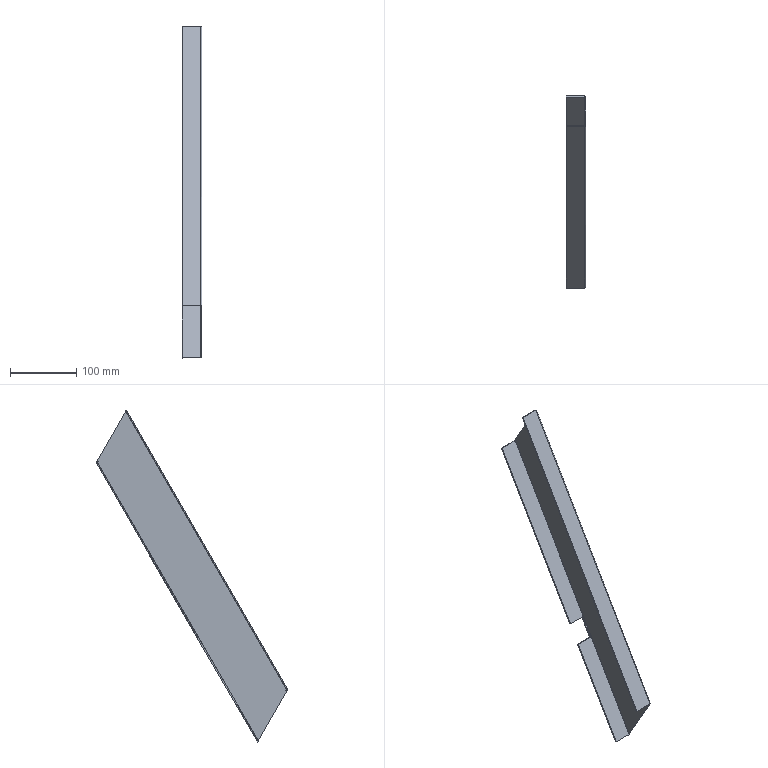Part | STEP file | Guard Rib 2 | 1 solid | 29 faces | box 30 x 290.188 x 502.62 mm | volume 129712 mm3 | plane 20 | cylinder 7 | spline 2 | commonest cylinder face diameters 1 x5 5 x2
STEP:
#1=CARTESIAN_POINT('',(-2.,-21.009,-479.727));
#2=VERTEX_POINT('',#1);
#3=CARTESIAN_POINT('',(-2.,-20.759,-478.794));
#4=VERTEX_POINT('',#3);
#5=CARTESIAN_POINT('',(-2.,-21.009,-479.227));
#6=DIRECTION('',(1.,0.,0.));
#7=DIRECTION('',(0.,0.,-1.));
#8=AXIS2_PLACEMENT_3D('',#5,#6,#7);
#9=CIRCLE('',#8,0.5);
#10=EDGE_CURVE('',#2,#4,#9,.T.);
#11=ORIENTED_EDGE('',*,*,#10,.F.);
#12=CARTESIAN_POINT('',(0.,-21.009,-479.727));
#13=VERTEX_POINT('',#12);
#14=CARTESIAN_POINT('',(-2.,-21.009,-479.727));
#15=DIRECTION('',(1.,0.,0.));
#16=VECTOR('',#15,1000.);
#17=LINE('',#14,#16);
#18=EDGE_CURVE('',#2,#13,#17,.T.);
#19=ORIENTED_EDGE('',*,*,#18,.T.);
#20=CARTESIAN_POINT('',(0.,-20.759,-478.794));
#21=VERTEX_POINT('',#20);
#22=CARTESIAN_POINT('',(0.,-21.009,-479.227));
#23=DIRECTION('',(-1.,0.,0.));
#24=DIRECTION('',(0.,0.,-1.));
#25=AXIS2_PLACEMENT_3D('',#22,#23,#24);
#26=CIRCLE('',#25,0.5);
#27=EDGE_CURVE('',#21,#13,#26,.T.);
#28=ORIENTED_EDGE('',*,*,#27,.F.);
#29=CARTESIAN_POINT('',(-2.,-20.759,-478.794));
#30=DIRECTION('',(1.,0.,0.));
#31=VECTOR('',#30,1000.);
#32=LINE('',#29,#31);
#33=EDGE_CURVE('',#4,#21,#32,.T.);
#34=ORIENTED_EDGE('',*,*,#33,.F.);
#35=EDGE_LOOP('',(#11,#19,#28,#34));
#36=FACE_OUTER_BOUND('',#35,.T.);
#37=CARTESIAN_POINT('',(-2.,-21.009,-479.227));
#38=DIRECTION('',(1.,0.,0.));
#39=DIRECTION('',(0.,0.,-1.));
#40=AXIS2_PLACEMENT_3D('',#37,#38,#39);
#41=CYLINDRICAL_SURFACE('',#40,0.5);
#42=ADVANCED_FACE('',(#36),#41,.F.);
#43=CARTESIAN_POINT('',(0.,-21.625,-478.294));
#44=VERTEX_POINT('',#43);
#45=CARTESIAN_POINT('',(0.,-21.625,-478.294));
#46=DIRECTION('',(0.,-0.866,0.5));
#47=VECTOR('',#46,1000.);
#48=LINE('',#45,#47);
#49=EDGE_CURVE('',#21,#44,#48,.T.);
#50=ORIENTED_EDGE('',*,*,#49,.F.);
#51=ORIENTED_EDGE('',*,*,#27,.T.);
#52=CARTESIAN_POINT('',(0.,-21.259,-479.66));
#53=VERTEX_POINT('',#52);
#54=CARTESIAN_POINT('',(0.,-21.009,-479.227));
#55=DIRECTION('',(-1.,0.,0.));
#56=DIRECTION('',(0.,0.,-1.));
#57=AXIS2_PLACEMENT_3D('',#54,#55,#56);
#58=CIRCLE('',#57,0.5);
#59=EDGE_CURVE('',#13,#53,#58,.T.);
#60=ORIENTED_EDGE('',*,*,#59,.T.);
#61=CARTESIAN_POINT('',(0.,-22.79,-478.776));
#62=VERTEX_POINT('',#61);
#63=CARTESIAN_POINT('',(0.,-22.79,-478.776));
#64=DIRECTION('',(0.,0.866,-0.5));
#65=VECTOR('',#64,1000.);
#66=LINE('',#63,#65);
#67=EDGE_CURVE('',#62,#53,#66,.T.);
#68=ORIENTED_EDGE('',*,*,#67,.F.);
#69=CARTESIAN_POINT('',(0.,20.955,-554.544));
#70=VERTEX_POINT('',#69);
#71=CARTESIAN_POINT('',(0.,20.955,-554.544));
#72=DIRECTION('',(0.,-0.5,0.866));
#73=VECTOR('',#72,1000.);
#74=LINE('',#71,#73);
#75=EDGE_CURVE('',#70,#62,#74,.T.);
#76=ORIENTED_EDGE('',*,*,#75,.F.);
#77=CARTESIAN_POINT('',(0.,264.233,-133.173));
#78=VERTEX_POINT('',#77);
#79=CARTESIAN_POINT('',(0.,264.233,-133.173));
#80=DIRECTION('',(0.,-0.5,-0.866));
#81=VECTOR('',#80,1000.);
#82=LINE('',#79,#81);
#83=EDGE_CURVE('',#78,#70,#82,.T.);
#84=ORIENTED_EDGE('',*,*,#83,.F.);
#85=CARTESIAN_POINT('',(0.,263.367,-132.673));
#86=VERTEX_POINT('',#85);
#87=CARTESIAN_POINT('',(0.,264.233,-133.173));
#88=DIRECTION('',(0.,0.866,-0.5));
#89=VECTOR('',#88,1000.);
#90=LINE('',#87,#89);
#91=EDGE_CURVE('',#86,#78,#90,.T.);
#92=ORIENTED_EDGE('',*,*,#91,.F.);
#93=CARTESIAN_POINT('',(0.,263.867,-131.807));
#94=VERTEX_POINT('',#93);
#95=CARTESIAN_POINT('',(0.,263.617,-132.24));
#96=DIRECTION('',(-1.,0.,0.));
#97=DIRECTION('',(0.,0.,-1.));
#98=AXIS2_PLACEMENT_3D('',#95,#96,#97);
#99=CIRCLE('',#98,0.5);
#100=EDGE_CURVE('',#86,#94,#99,.T.);
#101=ORIENTED_EDGE('',*,*,#100,.T.);
#102=CARTESIAN_POINT('',(0.,265.398,-132.691));
#103=VERTEX_POINT('',#102);
#104=CARTESIAN_POINT('',(0.,265.398,-132.691));
#105=DIRECTION('',(0.,-0.866,0.5));
#106=VECTOR('',#105,1000.);
#107=LINE('',#104,#106);
#108=EDGE_CURVE('',#103,#94,#107,.T.);
#109=ORIENTED_EDGE('',*,*,#108,.F.);
#110=CARTESIAN_POINT('',(0.,221.653,-56.923));
#111=VERTEX_POINT('',#110);
#112=CARTESIAN_POINT('',(0.,221.653,-56.923));
#113=DIRECTION('',(0.,0.5,-0.866));
#114=VECTOR('',#113,1000.);
#115=LINE('',#112,#114);
#116=EDGE_CURVE('',#111,#103,#115,.T.);
#117=ORIENTED_EDGE('',*,*,#116,.F.);
#118=CARTESIAN_POINT('',(0.,-21.625,-478.294));
#119=DIRECTION('',(0.,0.5,0.866));
#120=VECTOR('',#119,1000.);
#121=LINE('',#118,#120);
#122=EDGE_CURVE('',#44,#111,#121,.T.);
#123=ORIENTED_EDGE('',*,*,#122,.F.);
#124=EDGE_LOOP('',(#50,#51,#60,#68,#76,#84,#92,#101,#109,#117,#123));
#125=FACE_OUTER_BOUND('',#124,.T.);
#126=CARTESIAN_POINT('',(0.,0.,0.));
#127=DIRECTION('',(-1.,0.,0.));
#128=DIRECTION('',(0.,0.,1.));
#129=AXIS2_PLACEMENT_3D('',#126,#127,#128);
#130=PLANE('',#129);
#131=ADVANCED_FACE('',(#125),#130,.F.);
#132=CARTESIAN_POINT('',(-2.5,220.21,-54.423));
#133=VERTEX_POINT('',#132);
#134=CARTESIAN_POINT('',(-2.5,-23.79,-477.044));
#135=VERTEX_POINT('',#134);
#136=CARTESIAN_POINT('',(-2.5,220.21,-54.423));
#137=DIRECTION('',(0.,-0.5,-0.866));
#138=VECTOR('',#137,1000.);
#139=LINE('',#136,#138);
#140=EDGE_CURVE('',#133,#135,#139,.T.);
#141=ORIENTED_EDGE('',*,*,#140,.T.);
#142=CARTESIAN_POINT('',(-2.5,-21.625,-478.294));
#143=DIRECTION('',(0.,0.5,0.866));
#144=DIRECTION('',(0.,-0.866,0.5));
#145=AXIS2_PLACEMENT_3D('',#142,#143,#144);
#146=CIRCLE('',#145,2.5);
#147=EDGE_CURVE('',#135,#44,#146,.T.);
#148=ORIENTED_EDGE('',*,*,#147,.T.);
#149=ORIENTED_EDGE('',*,*,#122,.T.);
#150=CARTESIAN_POINT('',(0.,221.653,-56.923));
#151=CARTESIAN_POINT('',(0.,221.428,-56.653));
#152=CARTESIAN_POINT('',(-0.0634,221.21,-56.392));
#153=CARTESIAN_POINT('',(-0.2525,220.905,-56.005));
#154=CARTESIAN_POINT('',(-0.3297,220.81,-55.881));
#155=CARTESIAN_POINT('',(-0.5105,220.635,-55.642));
#156=CARTESIAN_POINT('',(-0.6149,220.555,-55.526));
#157=CARTESIAN_POINT('',(-0.8474,220.414,-55.305));
#158=CARTESIAN_POINT('',(-0.9735,220.354,-55.201));
#159=CARTESIAN_POINT('',(-1.244,220.257,-55.007));
#160=CARTESIAN_POINT('',(-1.391,220.219,-54.915));
#161=CARTESIAN_POINT('',(-1.693,220.17,-54.748));
#162=CARTESIAN_POINT('',(-1.849,220.159,-54.673));
#163=CARTESIAN_POINT('',(-2.17,220.164,-54.537));
#164=CARTESIAN_POINT('',(-2.335,220.18,-54.476));
#165=CARTESIAN_POINT('',(-2.5,220.21,-54.423));
#166=B_SPLINE_CURVE_WITH_KNOTS('',3,(#150,#151,#152,#153,#154,#155,#156,#157,#158,#159,#160,#161,#162,#163,#164,#165),.UNSPECIFIED.,.F.,.F.,(4,2,2,2,2,2,2,4),(0.,0.001038,0.001557,0.002076,0.002595,0.003114,0.003633,0.004151),.UNSPECIFIED.);
#167=EDGE_CURVE('',#111,#133,#166,.T.);
#168=ORIENTED_EDGE('',*,*,#167,.T.);
#169=EDGE_LOOP('',(#141,#148,#149,#168));
#170=FACE_OUTER_BOUND('',#169,.T.);
#171=CARTESIAN_POINT('',(-2.5,222.375,-55.673));
#172=DIRECTION('',(0.,0.5,0.866));
#173=DIRECTION('',(0.,-0.866,0.5));
#174=AXIS2_PLACEMENT_3D('',#171,#172,#173);
#175=CYLINDRICAL_SURFACE('',#174,2.5);
#176=ADVANCED_FACE('',(#170),#175,.T.);
#177=CARTESIAN_POINT('',(-2.,-21.259,-479.66));
#178=VERTEX_POINT('',#177);
#179=CARTESIAN_POINT('',(-2.,-21.259,-479.66));
#180=DIRECTION('',(-1.,0.,0.));
#181=VECTOR('',#180,1000.);
#182=LINE('',#179,#181);
#183=EDGE_CURVE('',#53,#178,#182,.T.);
#184=ORIENTED_EDGE('',*,*,#183,.T.);
#185=CARTESIAN_POINT('',(-2.,-22.79,-478.776));
#186=VERTEX_POINT('',#185);
#187=CARTESIAN_POINT('',(-2.,-21.259,-479.66));
#188=DIRECTION('',(0.,-0.866,0.5));
#189=VECTOR('',#188,1000.);
#190=LINE('',#187,#189);
#191=EDGE_CURVE('',#178,#186,#190,.T.);
#192=ORIENTED_EDGE('',*,*,#191,.T.);
#193=CARTESIAN_POINT('',(-2.,-22.79,-478.776));
#194=DIRECTION('',(1.,0.,0.));
#195=VECTOR('',#194,1000.);
#196=LINE('',#193,#195);
#197=EDGE_CURVE('',#186,#62,#196,.T.);
#198=ORIENTED_EDGE('',*,*,#197,.T.);
#199=ORIENTED_EDGE('',*,*,#67,.T.);
#200=EDGE_LOOP('',(#184,#192,#198,#199));
#201=FACE_OUTER_BOUND('',#200,.T.);
#202=CARTESIAN_POINT('',(-2.,-21.259,-479.66));
#203=DIRECTION('',(0.,0.5,0.866));
#204=DIRECTION('',(0.,-0.866,0.5));
#205=AXIS2_PLACEMENT_3D('',#202,#203,#204);
#206=PLANE('',#205);
#207=ADVANCED_FACE('',(#201),#206,.T.);
#208=CARTESIAN_POINT('',(-2.,20.955,-554.544));
#209=VERTEX_POINT('',#208);
#210=CARTESIAN_POINT('',(-2.,-23.79,-477.044));
#211=DIRECTION('',(0.,0.5,-0.866));
#212=VECTOR('',#211,1000.);
#213=LINE('',#210,#212);
#214=EDGE_CURVE('',#186,#209,#213,.T.);
#215=ORIENTED_EDGE('',*,*,#214,.T.);
#216=CARTESIAN_POINT('',(-2.,20.955,-554.544));
#217=DIRECTION('',(1.,0.,0.));
#218=VECTOR('',#217,1000.);
#219=LINE('',#216,#218);
#220=EDGE_CURVE('',#209,#70,#219,.T.);
#221=ORIENTED_EDGE('',*,*,#220,.T.);
#222=ORIENTED_EDGE('',*,*,#75,.T.);
#223=ORIENTED_EDGE('',*,*,#197,.F.);
#224=EDGE_LOOP('',(#215,#221,#222,#223));
#225=FACE_OUTER_BOUND('',#224,.T.);
#226=CARTESIAN_POINT('',(-2.,-23.79,-477.044));
#227=DIRECTION('',(0.,-0.866,-0.5));
#228=DIRECTION('',(0.,0.5,-0.866));
#229=AXIS2_PLACEMENT_3D('',#226,#227,#228);
#230=PLANE('',#229);
#231=ADVANCED_FACE('',(#225),#230,.T.);
#232=CARTESIAN_POINT('',(-2.5,22.398,-557.044));
#233=VERTEX_POINT('',#232);
#234=CARTESIAN_POINT('',(-2.5,266.398,-134.423));
#235=VERTEX_POINT('',#234);
#236=CARTESIAN_POINT('',(-2.5,22.398,-557.044));
#237=DIRECTION('',(0.,0.5,0.866));
#238=VECTOR('',#237,1000.);
#239=LINE('',#236,#238);
#240=EDGE_CURVE('',#233,#235,#239,.T.);
#241=ORIENTED_EDGE('',*,*,#240,.T.);
#242=CARTESIAN_POINT('',(-2.5,264.233,-133.173));
#243=DIRECTION('',(0.,-0.5,-0.866));
#244=DIRECTION('',(0.,0.866,-0.5));
#245=AXIS2_PLACEMENT_3D('',#242,#243,#244);
#246=CIRCLE('',#245,2.5);
#247=EDGE_CURVE('',#235,#78,#246,.T.);
#248=ORIENTED_EDGE('',*,*,#247,.T.);
#249=ORIENTED_EDGE('',*,*,#83,.T.);
#250=CARTESIAN_POINT('',(0.,20.955,-554.544));
#251=CARTESIAN_POINT('',(0.,21.18,-554.814));
#252=CARTESIAN_POINT('',(-0.0634,21.398,-555.075));
#253=CARTESIAN_POINT('',(-0.2525,21.703,-555.462));
#254=CARTESIAN_POINT('',(-0.3297,21.798,-555.586));
#255=CARTESIAN_POINT('',(-0.5105,21.973,-555.825));
#256=CARTESIAN_POINT('',(-0.6149,22.054,-555.941));
#257=CARTESIAN_POINT('',(-0.8474,22.195,-556.162));
#258=CARTESIAN_POINT('',(-0.9735,22.255,-556.265));
#259=CARTESIAN_POINT('',(-1.244,22.352,-556.46));
#260=CARTESIAN_POINT('',(-1.391,22.389,-556.552));
#261=CARTESIAN_POINT('',(-1.693,22.438,-556.719));
#262=CARTESIAN_POINT('',(-1.849,22.449,-556.794));
#263=CARTESIAN_POINT('',(-2.17,22.445,-556.93));
#264=CARTESIAN_POINT('',(-2.335,22.428,-556.991));
#265=CARTESIAN_POINT('',(-2.5,22.398,-557.044));
#266=B_SPLINE_CURVE_WITH_KNOTS('',3,(#250,#251,#252,#253,#254,#255,#256,#257,#258,#259,#260,#261,#262,#263,#264,#265),.UNSPECIFIED.,.F.,.F.,(4,2,2,2,2,2,2,4),(0.,0.001038,0.001557,0.002076,0.002595,0.003114,0.003633,0.004151),.UNSPECIFIED.);
#267=EDGE_CURVE('',#70,#233,#266,.T.);
#268=ORIENTED_EDGE('',*,*,#267,.T.);
#269=EDGE_LOOP('',(#241,#248,#249,#268));
#270=FACE_OUTER_BOUND('',#269,.T.);
#271=CARTESIAN_POINT('',(-2.5,20.233,-555.794));
#272=DIRECTION('',(0.,-0.5,-0.866));
#273=DIRECTION('',(0.,0.866,-0.5));
#274=AXIS2_PLACEMENT_3D('',#271,#272,#273);
#275=CYLINDRICAL_SURFACE('',#274,2.5);
#276=ADVANCED_FACE('',(#270),#275,.T.);
#277=CARTESIAN_POINT('',(-2.,263.867,-131.807));
#278=VERTEX_POINT('',#277);
#279=CARTESIAN_POINT('',(-2.,263.867,-131.807));
#280=DIRECTION('',(-1.,0.,0.));
#281=VECTOR('',#280,1000.);
#282=LINE('',#279,#281);
#283=EDGE_CURVE('',#94,#278,#282,.T.);
#284=ORIENTED_EDGE('',*,*,#283,.T.);
#285=CARTESIAN_POINT('',(-2.,265.398,-132.691));
#286=VERTEX_POINT('',#285);
#287=CARTESIAN_POINT('',(-2.,263.867,-131.807));
#288=DIRECTION('',(0.,0.866,-0.5));
#289=VECTOR('',#288,1000.);
#290=LINE('',#287,#289);
#291=EDGE_CURVE('',#278,#286,#290,.T.);
#292=ORIENTED_EDGE('',*,*,#291,.T.);
#293=CARTESIAN_POINT('',(-2.,265.398,-132.691));
#294=DIRECTION('',(1.,0.,0.));
#295=VECTOR('',#294,1000.);
#296=LINE('',#293,#295);
#297=EDGE_CURVE('',#286,#103,#296,.T.);
#298=ORIENTED_EDGE('',*,*,#297,.T.);
#299=ORIENTED_EDGE('',*,*,#108,.T.);
#300=EDGE_LOOP('',(#284,#292,#298,#299));
#301=FACE_OUTER_BOUND('',#300,.T.);
#302=CARTESIAN_POINT('',(-2.,263.867,-131.807));
#303=DIRECTION('',(0.,-0.5,-0.866));
#304=DIRECTION('',(0.,0.866,-0.5));
#305=AXIS2_PLACEMENT_3D('',#302,#303,#304);
#306=PLANE('',#305);
#307=ADVANCED_FACE('',(#301),#306,.T.);
#308=ORIENTED_EDGE('',*,*,#116,.T.);
#309=ORIENTED_EDGE('',*,*,#297,.F.);
#310=CARTESIAN_POINT('',(-2.,221.653,-56.923));
#311=VERTEX_POINT('',#310);
#312=CARTESIAN_POINT('',(-2.,220.21,-54.423));
#313=DIRECTION('',(0.,-0.5,0.866));
#314=VECTOR('',#313,1000.);
#315=LINE('',#312,#314);
#316=EDGE_CURVE('',#286,#311,#315,.T.);
#317=ORIENTED_EDGE('',*,*,#316,.T.);
#318=CARTESIAN_POINT('',(-2.,221.653,-56.923));
#319=DIRECTION('',(1.,0.,0.));
#320=VECTOR('',#319,1000.);
#321=LINE('',#318,#320);
#322=EDGE_CURVE('',#311,#111,#321,.T.);
#323=ORIENTED_EDGE('',*,*,#322,.T.);
#324=EDGE_LOOP('',(#308,#309,#317,#323));
#325=FACE_OUTER_BOUND('',#324,.T.);
#326=CARTESIAN_POINT('',(-2.,220.21,-54.423));
#327=DIRECTION('',(0.,0.866,0.5));
#328=DIRECTION('',(0.,-0.5,0.866));
#329=AXIS2_PLACEMENT_3D('',#326,#327,#328);
#330=PLANE('',#329);
#331=ADVANCED_FACE('',(#325),#330,.T.);
#332=CARTESIAN_POINT('',(-2.5,-22.058,-478.044));
#333=VERTEX_POINT('',#332);
#334=CARTESIAN_POINT('',(-2.,-21.625,-478.294));
#335=VERTEX_POINT('',#334);
#336=CARTESIAN_POINT('',(-2.5,-21.625,-478.294));
#337=DIRECTION('',(0.,0.5,0.866));
#338=DIRECTION('',(0.,-0.866,0.5));
#339=AXIS2_PLACEMENT_3D('',#336,#337,#338);
#340=CIRCLE('',#339,0.5);
#341=EDGE_CURVE('',#333,#335,#340,.T.);
#342=ORIENTED_EDGE('',*,*,#341,.T.);
#343=CARTESIAN_POINT('',(-2.,-20.759,-478.794));
#344=DIRECTION('',(0.,-0.866,0.5));
#345=VECTOR('',#344,1000.);
#346=LINE('',#343,#345);
#347=EDGE_CURVE('',#4,#335,#346,.T.);
#348=ORIENTED_EDGE('',*,*,#347,.F.);
#349=ORIENTED_EDGE('',*,*,#33,.T.);
#350=ORIENTED_EDGE('',*,*,#49,.T.);
#351=ORIENTED_EDGE('',*,*,#147,.F.);
#352=CARTESIAN_POINT('',(-30.,-23.79,-477.044));
#353=VERTEX_POINT('',#352);
#354=CARTESIAN_POINT('',(0.,-23.79,-477.044));
#355=DIRECTION('',(-1.,0.,0.));
#356=VECTOR('',#355,1000.);
#357=LINE('',#354,#356);
#358=EDGE_CURVE('',#135,#353,#357,.T.);
#359=ORIENTED_EDGE('',*,*,#358,.T.);
#360=CARTESIAN_POINT('',(-30.,-22.058,-478.044));
#361=VERTEX_POINT('',#360);
#362=CARTESIAN_POINT('',(-30.,-23.79,-477.044));
#363=DIRECTION('',(0.,0.866,-0.5));
#364=VECTOR('',#363,1000.);
#365=LINE('',#362,#364);
#366=EDGE_CURVE('',#353,#361,#365,.T.);
#367=ORIENTED_EDGE('',*,*,#366,.T.);
#368=CARTESIAN_POINT('',(-2.,-22.058,-478.044));
#369=DIRECTION('',(1.,0.,0.));
#370=VECTOR('',#369,1000.);
#371=LINE('',#368,#370);
#372=EDGE_CURVE('',#361,#333,#371,.T.);
#373=ORIENTED_EDGE('',*,*,#372,.T.);
#374=EDGE_LOOP('',(#342,#348,#349,#350,#351,#359,#367,#373));
#375=FACE_OUTER_BOUND('',#374,.T.);
#376=CARTESIAN_POINT('',(-2.5,-21.625,-478.294));
#377=DIRECTION('',(0.,-0.5,-0.866));
#378=DIRECTION('',(0.,0.866,-0.5));
#379=AXIS2_PLACEMENT_3D('',#376,#377,#378);
#380=PLANE('',#379);
#381=ADVANCED_FACE('',(#375),#380,.T.);
#382=CARTESIAN_POINT('',(-30.,220.21,-54.423));
#383=VERTEX_POINT('',#382);
#384=CARTESIAN_POINT('',(0.,220.21,-54.423));
#385=DIRECTION('',(1.,0.,0.));
#386=VECTOR('',#385,1000.);
#387=LINE('',#384,#386);
#388=EDGE_CURVE('',#383,#133,#387,.T.);
#389=ORIENTED_EDGE('',*,*,#388,.F.);
#390=CARTESIAN_POINT('',(-30.,188.724,-108.96));
#391=DIRECTION('',(0.,0.5,0.866));
#392=VECTOR('',#391,1000.);
#393=LINE('',#390,#392);
#394=EDGE_CURVE('',#353,#383,#393,.T.);
#395=ORIENTED_EDGE('',*,*,#394,.F.);
#396=ORIENTED_EDGE('',*,*,#358,.F.);
#397=ORIENTED_EDGE('',*,*,#140,.F.);
#398=EDGE_LOOP('',(#389,#395,#396,#397));
#399=FACE_OUTER_BOUND('',#398,.T.);
#400=CARTESIAN_POINT('',(0.,188.724,-108.96));
#401=DIRECTION('',(0.,0.866,-0.5));
#402=DIRECTION('',(0.,0.5,0.866));
#403=AXIS2_PLACEMENT_3D('',#400,#401,#402);
#404=PLANE('',#403);
#405=ADVANCED_FACE('',(#399),#404,.F.);
#406=CARTESIAN_POINT('',(-2.5,221.942,-55.423));
#407=VERTEX_POINT('',#406);
#408=CARTESIAN_POINT('',(-2.5,221.076,-54.923));
#409=DIRECTION('',(0.,0.866,-0.5));
#410=VECTOR('',#409,1000.);
#411=LINE('',#408,#410);
#412=EDGE_CURVE('',#133,#407,#411,.T.);
#413=ORIENTED_EDGE('',*,*,#412,.F.);
#414=ORIENTED_EDGE('',*,*,#167,.F.);
#415=ORIENTED_EDGE('',*,*,#322,.F.);
#416=CARTESIAN_POINT('',(-2.,221.653,-56.923));
#417=CARTESIAN_POINT('',(-2.,221.657,-56.785));
#418=CARTESIAN_POINT('',(-2.013,221.66,-56.649));
#419=CARTESIAN_POINT('',(-2.063,221.676,-56.382));
#420=CARTESIAN_POINT('',(-2.1,221.688,-56.249));
#421=CARTESIAN_POINT('',(-2.239,221.748,-55.866));
#422=CARTESIAN_POINT('',(-2.368,221.821,-55.633));
#423=CARTESIAN_POINT('',(-2.5,221.942,-55.423));
#424=B_SPLINE_CURVE_WITH_KNOTS('',3,(#416,#417,#418,#419,#420,#421,#422,#423),.UNSPECIFIED.,.F.,.F.,(4,2,2,4),(0.,0.0004085,0.0008171,0.001634),.UNSPECIFIED.);
#425=EDGE_CURVE('',#311,#407,#424,.T.);
#426=ORIENTED_EDGE('',*,*,#425,.T.);
#427=EDGE_LOOP('',(#413,#414,#415,#426));
#428=FACE_OUTER_BOUND('',#427,.T.);
#429=CARTESIAN_POINT('',(-2.5,220.193,-54.413));
#430=CARTESIAN_POINT('',(-2.17,220.133,-54.517));
#431=CARTESIAN_POINT('',(-1.84,220.129,-54.654));
#432=CARTESIAN_POINT('',(-1.231,220.228,-54.989));
#433=CARTESIAN_POINT('',(-0.9513,220.329,-55.186));
#434=CARTESIAN_POINT('',(-0.4848,220.613,-55.628));
#435=CARTESIAN_POINT('',(-0.2981,220.795,-55.872));
#436=CARTESIAN_POINT('',(-0.04559,221.203,-56.385));
#437=CARTESIAN_POINT('',(0.02,221.428,-56.654));
#438=CARTESIAN_POINT('',(0.02,221.653,-56.923));
#439=CARTESIAN_POINT('',(-2.5,220.21,-54.423));
#440=CARTESIAN_POINT('',(-2.173,220.15,-54.527));
#441=CARTESIAN_POINT('',(-1.846,220.146,-54.664));
#442=CARTESIAN_POINT('',(-1.241,220.243,-54.998));
#443=CARTESIAN_POINT('',(-0.9636,220.343,-55.194));
#444=CARTESIAN_POINT('',(-0.5008,220.624,-55.634));
#445=CARTESIAN_POINT('',(-0.3155,220.804,-55.877));
#446=CARTESIAN_POINT('',(-0.06507,221.207,-56.388));
#447=CARTESIAN_POINT('',(0.,221.43,-56.655));
#448=CARTESIAN_POINT('',(0.,221.653,-56.923));
#449=CARTESIAN_POINT('',(-2.5,221.942,-55.423));
#450=CARTESIAN_POINT('',(-2.435,221.882,-55.527));
#451=CARTESIAN_POINT('',(-2.369,221.833,-55.638));
#452=CARTESIAN_POINT('',(-2.248,221.756,-55.871));
#453=CARTESIAN_POINT('',(-2.193,221.728,-55.994));
#454=CARTESIAN_POINT('',(-2.1,221.688,-56.249));
#455=CARTESIAN_POINT('',(-2.063,221.676,-56.381));
#456=CARTESIAN_POINT('',(-2.013,221.66,-56.649));
#457=CARTESIAN_POINT('',(-2.,221.657,-56.786));
#458=CARTESIAN_POINT('',(-2.,221.653,-56.923));
#459=CARTESIAN_POINT('',(-2.5,221.96,-55.433));
#460=CARTESIAN_POINT('',(-2.437,221.9,-55.537));
#461=CARTESIAN_POINT('',(-2.374,221.85,-55.648));
#462=CARTESIAN_POINT('',(-2.258,221.772,-55.88));
#463=CARTESIAN_POINT('',(-2.205,221.742,-56.002));
#464=CARTESIAN_POINT('',(-2.116,221.699,-56.255));
#465=CARTESIAN_POINT('',(-2.081,221.685,-56.386));
#466=CARTESIAN_POINT('',(-2.033,221.665,-56.652));
#467=CARTESIAN_POINT('',(-2.02,221.659,-56.788));
#468=CARTESIAN_POINT('',(-2.02,221.653,-56.923));
#469=B_SPLINE_SURFACE_WITH_KNOTS('',1,3,((#429,#430,#431,#432,#433,#434,#435,#436,#437,#438),(#439,#440,#441,#442,#443,#444,#445,#446,#447,#448),(#449,#450,#451,#452,#453,#454,#455,#456,#457,#458),(#459,#460,#461,#462,#463,#464,#465,#466,#467,#468)),.UNSPECIFIED.,.F.,.F.,.F.,(2,1,1,2),(4,2,2,2,4),(-0.01,0.,1.,1.01),(0.,0.25,0.5,0.75,1.),.UNSPECIFIED.);
#470=ADVANCED_FACE('',(#428),#469,.F.);
#471=CARTESIAN_POINT('',(-2.,-21.009,-479.227));
#472=DIRECTION('',(1.,0.,0.));
#473=DIRECTION('',(0.,0.,-1.));
#474=AXIS2_PLACEMENT_3D('',#471,#472,#473);
#475=CIRCLE('',#474,0.5);
#476=EDGE_CURVE('',#178,#2,#475,.T.);
#477=ORIENTED_EDGE('',*,*,#476,.T.);
#478=ORIENTED_EDGE('',*,*,#10,.T.);
#479=ORIENTED_EDGE('',*,*,#347,.T.);
#480=CARTESIAN_POINT('',(-2.,-21.625,-478.294));
#481=DIRECTION('',(0.,0.5,0.866));
#482=VECTOR('',#481,1000.);
#483=LINE('',#480,#482);
#484=EDGE_CURVE('',#335,#311,#483,.T.);
#485=ORIENTED_EDGE('',*,*,#484,.T.);
#486=ORIENTED_EDGE('',*,*,#316,.F.);
#487=ORIENTED_EDGE('',*,*,#291,.F.);
#488=CARTESIAN_POINT('',(-2.,263.367,-132.673));
#489=VERTEX_POINT('',#488);
#490=CARTESIAN_POINT('',(-2.,263.617,-132.24));
#491=DIRECTION('',(1.,0.,0.));
#492=DIRECTION('',(0.,0.,-1.));
#493=AXIS2_PLACEMENT_3D('',#490,#491,#492);
#494=CIRCLE('',#493,0.5);
#495=EDGE_CURVE('',#278,#489,#494,.T.);
#496=ORIENTED_EDGE('',*,*,#495,.T.);
#497=CARTESIAN_POINT('',(-2.,264.233,-133.173));
#498=VERTEX_POINT('',#497);
#499=CARTESIAN_POINT('',(-2.,264.233,-133.173));
#500=DIRECTION('',(0.,-0.866,0.5));
#501=VECTOR('',#500,1000.);
#502=LINE('',#499,#501);
#503=EDGE_CURVE('',#498,#489,#502,.T.);
#504=ORIENTED_EDGE('',*,*,#503,.F.);
#505=CARTESIAN_POINT('',(-2.,264.233,-133.173));
#506=DIRECTION('',(0.,-0.5,-0.866));
#507=VECTOR('',#506,1000.);
#508=LINE('',#505,#507);
#509=EDGE_CURVE('',#498,#209,#508,.T.);
#510=ORIENTED_EDGE('',*,*,#509,.T.);
#511=ORIENTED_EDGE('',*,*,#214,.F.);
#512=ORIENTED_EDGE('',*,*,#191,.F.);
#513=EDGE_LOOP('',(#477,#478,#479,#485,#486,#487,#496,#504,#510,#511,#512));
#514=FACE_OUTER_BOUND('',#513,.T.);
#515=CARTESIAN_POINT('',(-2.,0.,0.));
#516=DIRECTION('',(-1.,0.,0.));
#517=DIRECTION('',(0.,0.,1.));
#518=AXIS2_PLACEMENT_3D('',#515,#516,#517);
#519=PLANE('',#518);
#520=ADVANCED_FACE('',(#514),#519,.T.);
#521=ORIENTED_EDGE('',*,*,#18,.F.);
#522=ORIENTED_EDGE('',*,*,#476,.F.);
#523=ORIENTED_EDGE('',*,*,#183,.F.);
#524=ORIENTED_EDGE('',*,*,#59,.F.);
#525=EDGE_LOOP('',(#521,#522,#523,#524));
#526=FACE_OUTER_BOUND('',#525,.T.);
#527=CARTESIAN_POINT('',(-2.,-21.009,-479.227));
#528=DIRECTION('',(1.,0.,0.));
#529=DIRECTION('',(0.,0.,-1.));
#530=AXIS2_PLACEMENT_3D('',#527,#528,#529);
#531=CYLINDRICAL_SURFACE('',#530,0.5);
#532=ADVANCED_FACE('',(#526),#531,.F.);
#533=CARTESIAN_POINT('',(-2.5,20.666,-556.044));
#534=VERTEX_POINT('',#533);
#535=CARTESIAN_POINT('',(-2.5,21.532,-556.544));
#536=DIRECTION('',(0.,-0.866,0.5));
#537=VECTOR('',#536,1000.);
#538=LINE('',#535,#537);
#539=EDGE_CURVE('',#233,#534,#538,.T.);
#540=ORIENTED_EDGE('',*,*,#539,.F.);
#541=ORIENTED_EDGE('',*,*,#267,.F.);
#542=ORIENTED_EDGE('',*,*,#220,.F.);
#543=CARTESIAN_POINT('',(-2.5,20.666,-556.044));
#544=CARTESIAN_POINT('',(-2.434,20.727,-555.939));
#545=CARTESIAN_POINT('',(-2.369,20.775,-555.829));
#546=CARTESIAN_POINT('',(-2.249,20.852,-555.596));
#547=CARTESIAN_POINT('',(-2.193,20.88,-555.473));
#548=CARTESIAN_POINT('',(-2.054,20.94,-555.09));
#549=CARTESIAN_POINT('',(-2.,20.948,-554.82));
#550=CARTESIAN_POINT('',(-2.,20.955,-554.544));
#551=B_SPLINE_CURVE_WITH_KNOTS('',3,(#543,#544,#545,#546,#547,#548,#549,#550),.UNSPECIFIED.,.F.,.F.,(4,2,2,4),(0.,0.0004085,0.0008171,0.001634),.UNSPECIFIED.);
#552=EDGE_CURVE('',#534,#209,#551,.T.);
#553=ORIENTED_EDGE('',*,*,#552,.F.);
#554=EDGE_LOOP('',(#540,#541,#542,#553));
#555=FACE_OUTER_BOUND('',#554,.T.);
#556=CARTESIAN_POINT('',(-2.5,22.415,-557.054));
#557=CARTESIAN_POINT('',(-2.17,22.476,-556.949));
#558=CARTESIAN_POINT('',(-1.84,22.479,-556.812));
#559=CARTESIAN_POINT('',(-1.231,22.381,-556.478));
#560=CARTESIAN_POINT('',(-0.9513,22.279,-556.28));
#561=CARTESIAN_POINT('',(-0.4848,21.995,-555.839));
#562=CARTESIAN_POINT('',(-0.2981,21.813,-555.595));
#563=CARTESIAN_POINT('',(-0.04559,21.406,-555.082));
#564=CARTESIAN_POINT('',(0.02,21.18,-554.813));
#565=CARTESIAN_POINT('',(0.02,20.955,-554.544));
#566=CARTESIAN_POINT('',(-2.5,22.398,-557.044));
#567=CARTESIAN_POINT('',(-2.173,22.458,-556.939));
#568=CARTESIAN_POINT('',(-1.846,22.462,-556.803));
#569=CARTESIAN_POINT('',(-1.241,22.365,-556.469));
#570=CARTESIAN_POINT('',(-0.9636,22.265,-556.272));
#571=CARTESIAN_POINT('',(-0.5008,21.985,-555.833));
#572=CARTESIAN_POINT('',(-0.3155,21.805,-555.59));
#573=CARTESIAN_POINT('',(-0.06507,21.401,-555.079));
#574=CARTESIAN_POINT('',(0.,21.178,-554.811));
#575=CARTESIAN_POINT('',(0.,20.955,-554.544));
#576=CARTESIAN_POINT('',(-2.5,20.666,-556.044));
#577=CARTESIAN_POINT('',(-2.435,20.726,-555.939));
#578=CARTESIAN_POINT('',(-2.369,20.775,-555.829));
#579=CARTESIAN_POINT('',(-2.248,20.852,-555.595));
#580=CARTESIAN_POINT('',(-2.193,20.88,-555.473));
#581=CARTESIAN_POINT('',(-2.1,20.92,-555.218));
#582=CARTESIAN_POINT('',(-2.063,20.932,-555.086));
#583=CARTESIAN_POINT('',(-2.013,20.948,-554.817));
#584=CARTESIAN_POINT('',(-2.,20.951,-554.68));
#585=CARTESIAN_POINT('',(-2.,20.955,-554.544));
#586=CARTESIAN_POINT('',(-2.5,20.649,-556.033));
#587=CARTESIAN_POINT('',(-2.437,20.709,-555.929));
#588=CARTESIAN_POINT('',(-2.374,20.758,-555.819));
#589=CARTESIAN_POINT('',(-2.258,20.837,-555.587));
#590=CARTESIAN_POINT('',(-2.205,20.866,-555.465));
#591=CARTESIAN_POINT('',(-2.116,20.909,-555.212));
#592=CARTESIAN_POINT('',(-2.081,20.923,-555.081));
#593=CARTESIAN_POINT('',(-2.033,20.943,-554.815));
#594=CARTESIAN_POINT('',(-2.02,20.949,-554.679));
#595=CARTESIAN_POINT('',(-2.02,20.955,-554.544));
#596=B_SPLINE_SURFACE_WITH_KNOTS('',1,3,((#556,#557,#558,#559,#560,#561,#562,#563,#564,#565),(#566,#567,#568,#569,#570,#571,#572,#573,#574,#575),(#576,#577,#578,#579,#580,#581,#582,#583,#584,#585),(#586,#587,#588,#589,#590,#591,#592,#593,#594,#595)),.UNSPECIFIED.,.F.,.F.,.F.,(2,1,1,2),(4,2,2,2,4),(-0.01,0.,1.,1.01),(0.,0.25,0.5,0.75,1.),.UNSPECIFIED.);
#597=ADVANCED_FACE('',(#555),#596,.F.);
#598=CARTESIAN_POINT('',(-2.5,264.666,-133.423));
#599=VERTEX_POINT('',#598);
#600=CARTESIAN_POINT('',(-2.5,264.233,-133.173));
#601=DIRECTION('',(0.,-0.5,-0.866));
#602=DIRECTION('',(0.,0.866,-0.5));
#603=AXIS2_PLACEMENT_3D('',#600,#601,#602);
#604=CIRCLE('',#603,0.5);
#605=EDGE_CURVE('',#599,#498,#604,.T.);
#606=ORIENTED_EDGE('',*,*,#605,.T.);
#607=ORIENTED_EDGE('',*,*,#503,.T.);
#608=CARTESIAN_POINT('',(-2.,263.367,-132.673));
#609=DIRECTION('',(1.,0.,0.));
#610=VECTOR('',#609,1000.);
#611=LINE('',#608,#610);
#612=EDGE_CURVE('',#489,#86,#611,.T.);
#613=ORIENTED_EDGE('',*,*,#612,.T.);
#614=ORIENTED_EDGE('',*,*,#91,.T.);
#615=ORIENTED_EDGE('',*,*,#247,.F.);
#616=CARTESIAN_POINT('',(-30.,266.398,-134.423));
#617=VERTEX_POINT('',#616);
#618=CARTESIAN_POINT('',(0.,266.398,-134.423));
#619=DIRECTION('',(1.,0.,0.));
#620=VECTOR('',#619,1000.);
#621=LINE('',#618,#620);
#622=EDGE_CURVE('',#617,#235,#621,.T.);
#623=ORIENTED_EDGE('',*,*,#622,.F.);
#624=CARTESIAN_POINT('',(-30.,264.666,-133.423));
#625=VERTEX_POINT('',#624);
#626=CARTESIAN_POINT('',(-30.,266.398,-134.423));
#627=DIRECTION('',(0.,-0.866,0.5));
#628=VECTOR('',#627,1000.);
#629=LINE('',#626,#628);
#630=EDGE_CURVE('',#617,#625,#629,.T.);
#631=ORIENTED_EDGE('',*,*,#630,.T.);
#632=CARTESIAN_POINT('',(-30.,264.666,-133.423));
#633=DIRECTION('',(1.,0.,0.));
#634=VECTOR('',#633,1000.);
#635=LINE('',#632,#634);
#636=EDGE_CURVE('',#625,#599,#635,.T.);
#637=ORIENTED_EDGE('',*,*,#636,.T.);
#638=EDGE_LOOP('',(#606,#607,#613,#614,#615,#623,#631,#637));
#639=FACE_OUTER_BOUND('',#638,.T.);
#640=CARTESIAN_POINT('',(-2.5,264.233,-133.173));
#641=DIRECTION('',(0.,0.5,0.866));
#642=DIRECTION('',(0.,-0.866,0.5));
#643=AXIS2_PLACEMENT_3D('',#640,#641,#642);
#644=PLANE('',#643);
#645=ADVANCED_FACE('',(#639),#644,.T.);
#646=CARTESIAN_POINT('',(-30.,22.398,-557.044));
#647=VERTEX_POINT('',#646);
#648=CARTESIAN_POINT('',(0.,22.398,-557.044));
#649=DIRECTION('',(-1.,0.,0.));
#650=VECTOR('',#649,1000.);
#651=LINE('',#648,#650);
#652=EDGE_CURVE('',#233,#647,#651,.T.);
#653=ORIENTED_EDGE('',*,*,#652,.T.);
#654=CARTESIAN_POINT('',(-30.,103.543,-416.496));
#655=VERTEX_POINT('',#654);
#656=CARTESIAN_POINT('',(-30.,258.006,-148.96));
#657=DIRECTION('',(0.,0.5,0.866));
#658=VECTOR('',#657,1000.);
#659=LINE('',#656,#658);
#660=EDGE_CURVE('',#647,#655,#659,.T.);
#661=ORIENTED_EDGE('',*,*,#660,.T.);
#662=CARTESIAN_POINT('',(-4.,103.543,-416.496));
#663=VERTEX_POINT('',#662);
#664=CARTESIAN_POINT('',(0.,103.543,-416.496));
#665=DIRECTION('',(1.,0.,0.));
#666=VECTOR('',#665,1000.);
#667=LINE('',#664,#666);
#668=EDGE_CURVE('',#655,#663,#667,.T.);
#669=ORIENTED_EDGE('',*,*,#668,.T.);
#670=CARTESIAN_POINT('',(-4.,120.429,-387.25));
#671=VERTEX_POINT('',#670);
#672=CARTESIAN_POINT('',(-4.,258.006,-148.96));
#673=DIRECTION('',(0.,0.5,0.866));
#674=VECTOR('',#673,1000.);
#675=LINE('',#672,#674);
#676=EDGE_CURVE('',#663,#671,#675,.T.);
#677=ORIENTED_EDGE('',*,*,#676,.T.);
#678=CARTESIAN_POINT('',(-30.,120.429,-387.25));
#679=VERTEX_POINT('',#678);
#680=CARTESIAN_POINT('',(0.,120.429,-387.25));
#681=DIRECTION('',(-1.,0.,0.));
#682=VECTOR('',#681,1000.);
#683=LINE('',#680,#682);
#684=EDGE_CURVE('',#671,#679,#683,.T.);
#685=ORIENTED_EDGE('',*,*,#684,.T.);
#686=CARTESIAN_POINT('',(-30.,258.006,-148.96));
#687=DIRECTION('',(0.,0.5,0.866));
#688=VECTOR('',#687,1000.);
#689=LINE('',#686,#688);
#690=EDGE_CURVE('',#679,#617,#689,.T.);
#691=ORIENTED_EDGE('',*,*,#690,.T.);
#692=ORIENTED_EDGE('',*,*,#622,.T.);
#693=ORIENTED_EDGE('',*,*,#240,.F.);
#694=EDGE_LOOP('',(#653,#661,#669,#677,#685,#691,#692,#693));
#695=FACE_OUTER_BOUND('',#694,.T.);
#696=CARTESIAN_POINT('',(0.,258.006,-148.96));
#697=DIRECTION('',(0.,0.866,-0.5));
#698=DIRECTION('',(0.,0.5,0.866));
#699=AXIS2_PLACEMENT_3D('',#696,#697,#698);
#700=PLANE('',#699);
#701=ADVANCED_FACE('',(#695),#700,.T.);
#702=ORIENTED_EDGE('',*,*,#100,.F.);
#703=ORIENTED_EDGE('',*,*,#612,.F.);
#704=ORIENTED_EDGE('',*,*,#495,.F.);
#705=ORIENTED_EDGE('',*,*,#283,.F.);
#706=EDGE_LOOP('',(#702,#703,#704,#705));
#707=FACE_OUTER_BOUND('',#706,.T.);
#708=CARTESIAN_POINT('',(-2.,263.617,-132.24));
#709=DIRECTION('',(1.,0.,0.));
#710=DIRECTION('',(0.,0.,-1.));
#711=AXIS2_PLACEMENT_3D('',#708,#709,#710);
#712=CYLINDRICAL_SURFACE('',#711,0.5);
#713=ADVANCED_FACE('',(#707),#712,.F.);
#714=CARTESIAN_POINT('',(-30.,221.942,-55.423));
#715=VERTEX_POINT('',#714);
#716=CARTESIAN_POINT('',(-30.,221.942,-55.423));
#717=DIRECTION('',(-1.,0.,0.));
#718=VECTOR('',#717,1000.);
#719=LINE('',#716,#718);
#720=EDGE_CURVE('',#407,#715,#719,.T.);
#721=ORIENTED_EDGE('',*,*,#720,.T.);
#722=CARTESIAN_POINT('',(-30.,220.21,-54.423));
#723=DIRECTION('',(0.,-0.866,0.5));
#724=VECTOR('',#723,1000.);
#725=LINE('',#722,#724);
#726=EDGE_CURVE('',#715,#383,#725,.T.);
#727=ORIENTED_EDGE('',*,*,#726,.T.);
#728=ORIENTED_EDGE('',*,*,#388,.T.);
#729=ORIENTED_EDGE('',*,*,#412,.T.);
#730=EDGE_LOOP('',(#721,#727,#728,#729));
#731=FACE_OUTER_BOUND('',#730,.T.);
#732=CARTESIAN_POINT('',(-30.,220.21,-54.423));
#733=DIRECTION('',(0.,0.5,0.866));
#734=DIRECTION('',(0.,-0.866,0.5));
#735=AXIS2_PLACEMENT_3D('',#732,#733,#734);
#736=PLANE('',#735);
#737=ADVANCED_FACE('',(#731),#736,.T.);
#738=ORIENTED_EDGE('',*,*,#394,.T.);
#739=ORIENTED_EDGE('',*,*,#726,.F.);
#740=CARTESIAN_POINT('',(-30.,221.942,-55.423));
#741=DIRECTION('',(0.,-0.5,-0.866));
#742=VECTOR('',#741,1000.);
#743=LINE('',#740,#742);
#744=EDGE_CURVE('',#715,#361,#743,.T.);
#745=ORIENTED_EDGE('',*,*,#744,.T.);
#746=ORIENTED_EDGE('',*,*,#366,.F.);
#747=EDGE_LOOP('',(#738,#739,#745,#746));
#748=FACE_OUTER_BOUND('',#747,.T.);
#749=CARTESIAN_POINT('',(-30.,-23.79,-477.044));
#750=DIRECTION('',(-1.,0.,0.));
#751=DIRECTION('',(0.,-1.,0.));
#752=AXIS2_PLACEMENT_3D('',#749,#750,#751);
#753=PLANE('',#752);
#754=ADVANCED_FACE('',(#748),#753,.T.);
#755=ORIENTED_EDGE('',*,*,#605,.F.);
#756=CARTESIAN_POINT('',(-2.5,20.666,-556.044));
#757=DIRECTION('',(0.,0.5,0.866));
#758=VECTOR('',#757,1000.);
#759=LINE('',#756,#758);
#760=EDGE_CURVE('',#534,#599,#759,.T.);
#761=ORIENTED_EDGE('',*,*,#760,.F.);
#762=ORIENTED_EDGE('',*,*,#552,.T.);
#763=ORIENTED_EDGE('',*,*,#509,.F.);
#764=EDGE_LOOP('',(#755,#761,#762,#763));
#765=FACE_OUTER_BOUND('',#764,.T.);
#766=CARTESIAN_POINT('',(-2.5,20.233,-555.794));
#767=DIRECTION('',(0.,-0.5,-0.866));
#768=DIRECTION('',(0.,0.866,-0.5));
#769=AXIS2_PLACEMENT_3D('',#766,#767,#768);
#770=CYLINDRICAL_SURFACE('',#769,0.5);
#771=ADVANCED_FACE('',(#765),#770,.F.);
#772=ORIENTED_EDGE('',*,*,#341,.F.);
#773=CARTESIAN_POINT('',(-2.5,221.942,-55.423));
#774=DIRECTION('',(0.,-0.5,-0.866));
#775=VECTOR('',#774,1000.);
#776=LINE('',#773,#775);
#777=EDGE_CURVE('',#407,#333,#776,.T.);
#778=ORIENTED_EDGE('',*,*,#777,.F.);
#779=ORIENTED_EDGE('',*,*,#425,.F.);
#780=ORIENTED_EDGE('',*,*,#484,.F.);
#781=EDGE_LOOP('',(#772,#778,#779,#780));
#782=FACE_OUTER_BOUND('',#781,.T.);
#783=CARTESIAN_POINT('',(-2.5,222.375,-55.673));
#784=DIRECTION('',(0.,0.5,0.866));
#785=DIRECTION('',(0.,-0.866,0.5));
#786=AXIS2_PLACEMENT_3D('',#783,#784,#785);
#787=CYLINDRICAL_SURFACE('',#786,0.5);
#788=ADVANCED_FACE('',(#782),#787,.F.);
#789=CARTESIAN_POINT('',(-30.,20.666,-556.044));
#790=VERTEX_POINT('',#789);
#791=CARTESIAN_POINT('',(-2.,20.666,-556.044));
#792=DIRECTION('',(-1.,0.,0.));
#793=VECTOR('',#792,1000.);
#794=LINE('',#791,#793);
#795=EDGE_CURVE('',#534,#790,#794,.T.);
#796=ORIENTED_EDGE('',*,*,#795,.T.);
#797=CARTESIAN_POINT('',(-30.,22.398,-557.044));
#798=DIRECTION('',(0.,0.866,-0.5));
#799=VECTOR('',#798,1000.);
#800=LINE('',#797,#799);
#801=EDGE_CURVE('',#790,#647,#800,.T.);
#802=ORIENTED_EDGE('',*,*,#801,.T.);
#803=ORIENTED_EDGE('',*,*,#652,.F.);
#804=ORIENTED_EDGE('',*,*,#539,.T.);
#805=EDGE_LOOP('',(#796,#802,#803,#804));
#806=FACE_OUTER_BOUND('',#805,.T.);
#807=CARTESIAN_POINT('',(-2.,22.398,-557.044));
#808=DIRECTION('',(0.,-0.5,-0.866));
#809=DIRECTION('',(0.,0.866,-0.5));
#810=AXIS2_PLACEMENT_3D('',#807,#808,#809);
#811=PLANE('',#810);
#812=ADVANCED_FACE('',(#806),#811,.T.);
#813=ORIENTED_EDGE('',*,*,#801,.F.);
#814=CARTESIAN_POINT('',(-30.,101.811,-415.496));
#815=VERTEX_POINT('',#814);
#816=CARTESIAN_POINT('',(-30.,20.666,-556.044));
#817=DIRECTION('',(0.,0.5,0.866));
#818=VECTOR('',#817,1000.);
#819=LINE('',#816,#818);
#820=EDGE_CURVE('',#790,#815,#819,.T.);
#821=ORIENTED_EDGE('',*,*,#820,.T.);
#822=CARTESIAN_POINT('',(-30.,101.811,-415.496));
#823=DIRECTION('',(0.,0.866,-0.5));
#824=VECTOR('',#823,1000.);
#825=LINE('',#822,#824);
#826=EDGE_CURVE('',#815,#655,#825,.T.);
#827=ORIENTED_EDGE('',*,*,#826,.T.);
#828=ORIENTED_EDGE('',*,*,#660,.F.);
#829=EDGE_LOOP('',(#813,#821,#827,#828));
#830=FACE_OUTER_BOUND('',#829,.T.);
#831=CARTESIAN_POINT('',(-30.,22.398,-557.044));
#832=DIRECTION('',(-1.,0.,0.));
#833=DIRECTION('',(0.,-1.,0.));
#834=AXIS2_PLACEMENT_3D('',#831,#832,#833);
#835=PLANE('',#834);
#836=ADVANCED_FACE('',(#830),#835,.T.);
#837=ORIENTED_EDGE('',*,*,#630,.F.);
#838=ORIENTED_EDGE('',*,*,#690,.F.);
#839=CARTESIAN_POINT('',(-30.,118.696,-386.25));
#840=VERTEX_POINT('',#839);
#841=CARTESIAN_POINT('',(-30.,120.429,-387.25));
#842=DIRECTION('',(0.,-0.866,0.5));
#843=VECTOR('',#842,1000.);
#844=LINE('',#841,#843);
#845=EDGE_CURVE('',#679,#840,#844,.T.);
#846=ORIENTED_EDGE('',*,*,#845,.T.);
#847=CARTESIAN_POINT('',(-30.,118.696,-386.25));
#848=DIRECTION('',(0.,0.5,0.866));
#849=VECTOR('',#848,1000.);
#850=LINE('',#847,#849);
#851=EDGE_CURVE('',#840,#625,#850,.T.);
#852=ORIENTED_EDGE('',*,*,#851,.T.);
#853=EDGE_LOOP('',(#837,#838,#846,#852));
#854=FACE_OUTER_BOUND('',#853,.T.);
#855=CARTESIAN_POINT('',(-30.,22.398,-557.044));
#856=DIRECTION('',(-1.,0.,0.));
#857=DIRECTION('',(0.,-1.,0.));
#858=AXIS2_PLACEMENT_3D('',#855,#856,#857);
#859=PLANE('',#858);
#860=ADVANCED_FACE('',(#854),#859,.T.);
#861=ORIENTED_EDGE('',*,*,#684,.F.);
#862=CARTESIAN_POINT('',(-4.,118.696,-386.25));
#863=VERTEX_POINT('',#862);
#864=CARTESIAN_POINT('',(-4.,111.768,-382.25));
#865=DIRECTION('',(0.,0.866,-0.5));
#866=VECTOR('',#865,1000.);
#867=LINE('',#864,#866);
#868=EDGE_CURVE('',#863,#671,#867,.T.);
#869=ORIENTED_EDGE('',*,*,#868,.F.);
#870=CARTESIAN_POINT('',(-4.,118.696,-386.25));
#871=DIRECTION('',(1.,0.,0.));
#872=VECTOR('',#871,1000.);
#873=LINE('',#870,#872);
#874=EDGE_CURVE('',#840,#863,#873,.T.);
#875=ORIENTED_EDGE('',*,*,#874,.F.);
#876=ORIENTED_EDGE('',*,*,#845,.F.);
#877=EDGE_LOOP('',(#861,#869,#875,#876));
#878=FACE_OUTER_BOUND('',#877,.T.);
#879=CARTESIAN_POINT('',(-4.,111.768,-382.25));
#880=DIRECTION('',(0.,0.5,0.866));
#881=DIRECTION('',(0.,-0.866,0.5));
#882=AXIS2_PLACEMENT_3D('',#879,#880,#881);
#883=PLANE('',#882);
#884=ADVANCED_FACE('',(#878),#883,.F.);
#885=ORIENTED_EDGE('',*,*,#676,.F.);
#886=CARTESIAN_POINT('',(-4.,101.811,-415.496));
#887=VERTEX_POINT('',#886);
#888=CARTESIAN_POINT('',(-4.,101.811,-415.496));
#889=DIRECTION('',(0.,0.866,-0.5));
#890=VECTOR('',#889,1000.);
#891=LINE('',#888,#890);
#892=EDGE_CURVE('',#887,#663,#891,.T.);
#893=ORIENTED_EDGE('',*,*,#892,.F.);
#894=CARTESIAN_POINT('',(-4.,118.696,-386.25));
#895=DIRECTION('',(0.,-0.5,-0.866));
#896=VECTOR('',#895,1000.);
#897=LINE('',#894,#896);
#898=EDGE_CURVE('',#863,#887,#897,.T.);
#899=ORIENTED_EDGE('',*,*,#898,.F.);
#900=ORIENTED_EDGE('',*,*,#868,.T.);
#901=EDGE_LOOP('',(#885,#893,#899,#900));
#902=FACE_OUTER_BOUND('',#901,.T.);
#903=CARTESIAN_POINT('',(-4.,94.883,-411.496));
#904=DIRECTION('',(1.,0.,0.));
#905=DIRECTION('',(0.,1.,0.));
#906=AXIS2_PLACEMENT_3D('',#903,#904,#905);
#907=PLANE('',#906);
#908=ADVANCED_FACE('',(#902),#907,.F.);
#909=ORIENTED_EDGE('',*,*,#668,.F.);
#910=ORIENTED_EDGE('',*,*,#826,.F.);
#911=CARTESIAN_POINT('',(-4.,101.811,-415.496));
#912=DIRECTION('',(-1.,0.,0.));
#913=VECTOR('',#912,1000.);
#914=LINE('',#911,#913);
#915=EDGE_CURVE('',#887,#815,#914,.T.);
#916=ORIENTED_EDGE('',*,*,#915,.F.);
#917=ORIENTED_EDGE('',*,*,#892,.T.);
#918=EDGE_LOOP('',(#909,#910,#916,#917));
#919=FACE_OUTER_BOUND('',#918,.T.);
#920=CARTESIAN_POINT('',(-4.,94.883,-411.496));
#921=DIRECTION('',(0.,-0.5,-0.866));
#922=DIRECTION('',(0.,0.866,-0.5));
#923=AXIS2_PLACEMENT_3D('',#920,#921,#922);
#924=PLANE('',#923);
#925=ADVANCED_FACE('',(#919),#924,.F.);
#926=ORIENTED_EDGE('',*,*,#372,.F.);
#927=ORIENTED_EDGE('',*,*,#744,.F.);
#928=ORIENTED_EDGE('',*,*,#720,.F.);
#929=ORIENTED_EDGE('',*,*,#777,.T.);
#930=EDGE_LOOP('',(#926,#927,#928,#929));
#931=FACE_OUTER_BOUND('',#930,.T.);
#932=CARTESIAN_POINT('',(0.,190.456,-109.96));
#933=DIRECTION('',(0.,0.866,-0.5));
#934=DIRECTION('',(0.,0.5,0.866));
#935=AXIS2_PLACEMENT_3D('',#932,#933,#934);
#936=PLANE('',#935);
#937=ADVANCED_FACE('',(#931),#936,.T.);
#938=ORIENTED_EDGE('',*,*,#915,.T.);
#939=ORIENTED_EDGE('',*,*,#820,.F.);
#940=ORIENTED_EDGE('',*,*,#795,.F.);
#941=ORIENTED_EDGE('',*,*,#760,.T.);
#942=ORIENTED_EDGE('',*,*,#636,.F.);
#943=ORIENTED_EDGE('',*,*,#851,.F.);
#944=ORIENTED_EDGE('',*,*,#874,.T.);
#945=ORIENTED_EDGE('',*,*,#898,.T.);
#946=EDGE_LOOP('',(#938,#939,#940,#941,#942,#943,#944,#945));
#947=FACE_OUTER_BOUND('',#946,.T.);
#948=CARTESIAN_POINT('',(0.,256.274,-147.96));
#949=DIRECTION('',(0.,0.866,-0.5));
#950=DIRECTION('',(0.,0.5,0.866));
#951=AXIS2_PLACEMENT_3D('',#948,#949,#950);
#952=PLANE('',#951);
#953=ADVANCED_FACE('',(#947),#952,.F.);
#954=CLOSED_SHELL('',(#42,#131,#176,#207,#231,#276,#307,#331,#381,#405,#470,#520,#532,#597,#645,#701,#713,#737,#754,#771,#788,#812,#836,#860,#884,#908,#925,#937,#953));
#955=MANIFOLD_SOLID_BREP('',#954);
#956=CARTESIAN_POINT('',(0.,0.,0.));
#957=DIRECTION('',(0.,0.,1.));
#958=DIRECTION('',(1.,0.,0.));
#959=AXIS2_PLACEMENT_3D('',#956,#957,#958);
#960=(LENGTH_UNIT()NAMED_UNIT(*)SI_UNIT(.MILLI.,.METRE.));
#961=UNCERTAINTY_MEASURE_WITH_UNIT(LENGTH_MEASURE(0.00001),#960,'','');
#962=(NAMED_UNIT(*)PLANE_ANGLE_UNIT()SI_UNIT($,.RADIAN.));
#963=(NAMED_UNIT(*)SI_UNIT($,.STERADIAN.)SOLID_ANGLE_UNIT());
#964=(GEOMETRIC_REPRESENTATION_CONTEXT(3)GLOBAL_UNCERTAINTY_ASSIGNED_CONTEXT((#961))GLOBAL_UNIT_ASSIGNED_CONTEXT((#960,#962,#963))REPRESENTATION_CONTEXT('',''));
#965=ADVANCED_BREP_SHAPE_REPRESENTATION('',(#955,#959),#964);